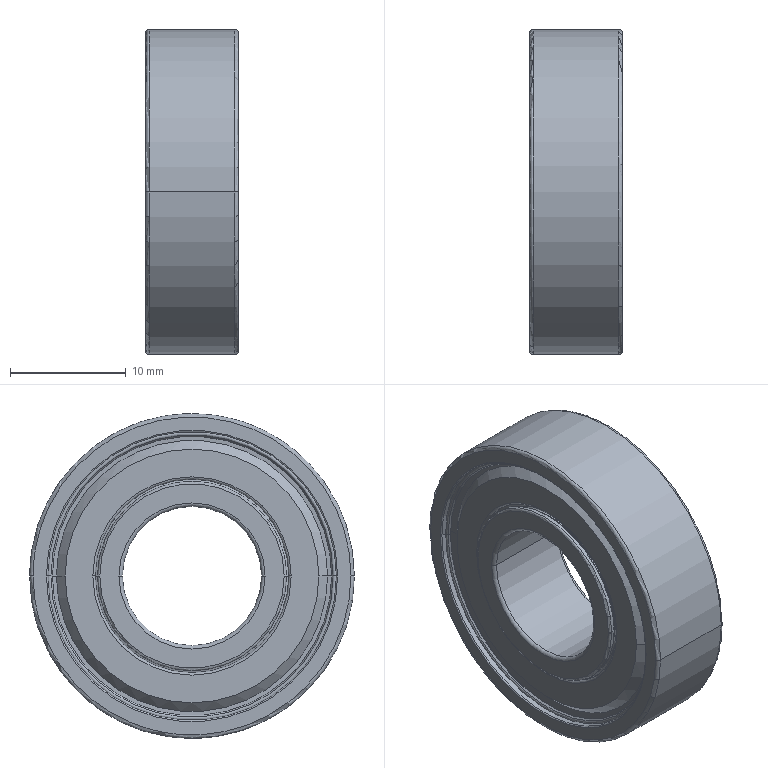Part | SolidWorks | features BaseBody 1 | 1 solid | 80 faces | box 8 x 28 x 28 mm | volume 3240 mm3 | torus 30 | cone 24 | cylinder 18 | plane 8 | commonest cylinder face diameters 17.5 x4 12 x2 15.5 x2 16.3 x2 16.7 x2 17.1 x2